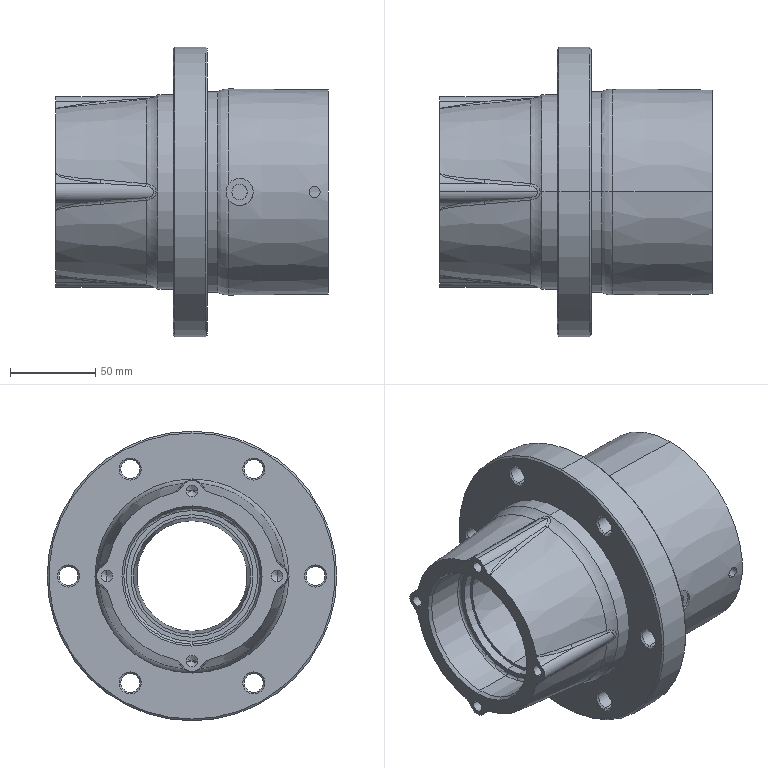Part | SolidWorks | features Chamfer 3, Fillet 3, Draft 2, RevCut 2, Boss 1, CirPattern 1, Cut 1, HoleWzd 1, Revolution 1 | 1 solid | 153 faces | box 160 x 170 x 170 mm | volume 858037 mm3 | cylinder 55 | cone 50 | spline 28 | torus 10 | plane 10 | commonest cylinder face diameters 11 x12 6.8 x8 20 x8 12 x5 6.5 x2 9 x2